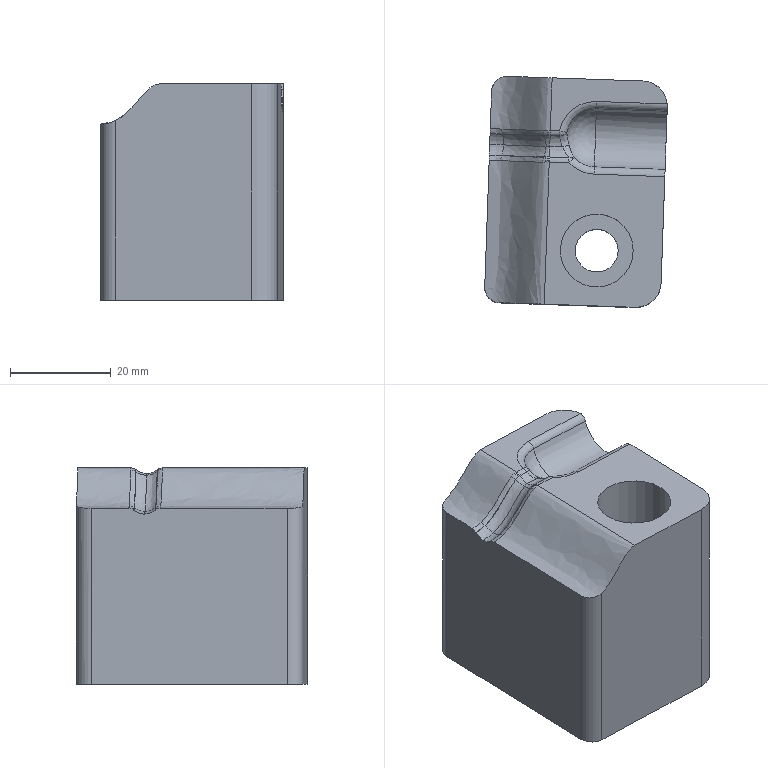Part | NX | features DIE-49 2 | 1 solid | 55 faces | box 36.275 x 45.92 x 43 mm | volume 60072 mm3 | spline 29 | cylinder 11 | plane 9 | torus 3 | sphere 3 | commonest cylinder face diameters 3 x4 6 x2 10 x2 8.506 x1 12 x1 14.5 x1